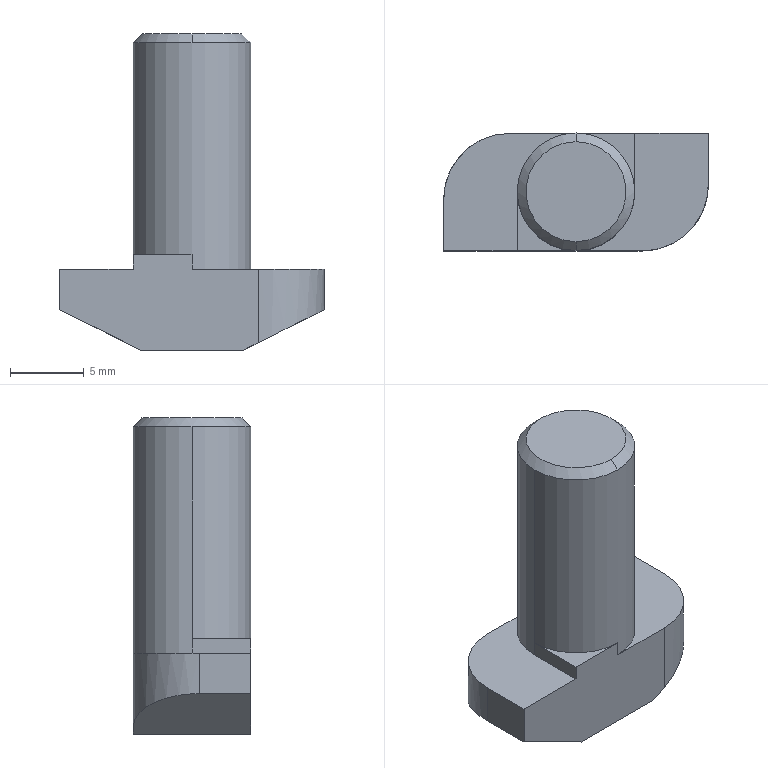Part | STEP file | LE-TS-M8X16-40_PN_0008 | 1 solid | 20 faces | box 18 x 8 x 21.5 mm | volume 1450 mm3 | plane 14 | cylinder 4 | cone 2 | commonest cylinder face diameters 8 x2 9 x2
STEP:
#1=CARTESIAN_POINT('',(0.,4.,15.4));
#2=VERTEX_POINT('',#1);
#3=CARTESIAN_POINT('',(4.,0.,15.4));
#4=VERTEX_POINT('',#3);
#5=CARTESIAN_POINT('',(0.,0.,15.4));
#6=DIRECTION('',(0.,0.,-1.));
#7=DIRECTION('',(-1.,0.,0.));
#8=AXIS2_PLACEMENT_3D('',#5,#6,#7);
#9=CIRCLE('',#8,4.);
#10=EDGE_CURVE('',#2,#4,#9,.T.);
#11=ORIENTED_EDGE('',*,*,#10,.T.);
#12=CARTESIAN_POINT('',(4.,0.,1.));
#13=VERTEX_POINT('',#12);
#14=CARTESIAN_POINT('',(4.,0.,1.));
#15=DIRECTION('',(0.,0.,-1.));
#16=VECTOR('',#15,1000.);
#17=LINE('',#14,#16);
#18=EDGE_CURVE('',#4,#13,#17,.T.);
#19=ORIENTED_EDGE('',*,*,#18,.T.);
#20=CARTESIAN_POINT('',(0.,4.,1.));
#21=VERTEX_POINT('',#20);
#22=CARTESIAN_POINT('',(0.,0.,1.));
#23=DIRECTION('',(0.,0.,1.));
#24=DIRECTION('',(-1.,0.,0.));
#25=AXIS2_PLACEMENT_3D('',#22,#23,#24);
#26=CIRCLE('',#25,4.);
#27=EDGE_CURVE('',#13,#21,#26,.T.);
#28=ORIENTED_EDGE('',*,*,#27,.T.);
#29=CARTESIAN_POINT('',(0.,4.,0.));
#30=VERTEX_POINT('',#29);
#31=CARTESIAN_POINT('',(0.,4.,0.));
#32=DIRECTION('',(0.,0.,-1.));
#33=VECTOR('',#32,1000.);
#34=LINE('',#31,#33);
#35=EDGE_CURVE('',#21,#30,#34,.T.);
#36=ORIENTED_EDGE('',*,*,#35,.T.);
#37=CARTESIAN_POINT('',(-4.,0.,0.));
#38=VERTEX_POINT('',#37);
#39=CARTESIAN_POINT('',(0.,0.,0.));
#40=DIRECTION('',(0.,0.,1.));
#41=DIRECTION('',(-1.,0.,0.));
#42=AXIS2_PLACEMENT_3D('',#39,#40,#41);
#43=CIRCLE('',#42,4.);
#44=EDGE_CURVE('',#30,#38,#43,.T.);
#45=ORIENTED_EDGE('',*,*,#44,.T.);
#46=CARTESIAN_POINT('',(-4.,0.,1.));
#47=VERTEX_POINT('',#46);
#48=CARTESIAN_POINT('',(-4.,0.,1.));
#49=DIRECTION('',(0.,0.,1.));
#50=VECTOR('',#49,1000.);
#51=LINE('',#48,#50);
#52=EDGE_CURVE('',#38,#47,#51,.T.);
#53=ORIENTED_EDGE('',*,*,#52,.T.);
#54=CARTESIAN_POINT('',(-4.,0.,15.4));
#55=VERTEX_POINT('',#54);
#56=CARTESIAN_POINT('',(-4.,0.,1.));
#57=DIRECTION('',(0.,0.,-1.));
#58=VECTOR('',#57,1000.);
#59=LINE('',#56,#58);
#60=EDGE_CURVE('',#55,#47,#59,.T.);
#61=ORIENTED_EDGE('',*,*,#60,.F.);
#62=CARTESIAN_POINT('',(0.,0.,15.4));
#63=DIRECTION('',(0.,0.,-1.));
#64=DIRECTION('',(-1.,0.,0.));
#65=AXIS2_PLACEMENT_3D('',#62,#63,#64);
#66=CIRCLE('',#65,4.);
#67=EDGE_CURVE('',#55,#2,#66,.T.);
#68=ORIENTED_EDGE('',*,*,#67,.T.);
#69=EDGE_LOOP('',(#11,#19,#28,#36,#45,#53,#61,#68));
#70=FACE_OUTER_BOUND('',#69,.T.);
#71=CARTESIAN_POINT('',(0.,0.,1.));
#72=DIRECTION('',(0.,0.,-1.));
#73=DIRECTION('',(-1.,0.,0.));
#74=AXIS2_PLACEMENT_3D('',#71,#72,#73);
#75=CYLINDRICAL_SURFACE('',#74,4.);
#76=ADVANCED_FACE('',(#70),#75,.T.);
#77=CARTESIAN_POINT('',(0.,3.4,16.));
#78=VERTEX_POINT('',#77);
#79=CARTESIAN_POINT('',(0.,-3.4,16.));
#80=VERTEX_POINT('',#79);
#81=CARTESIAN_POINT('',(0.,0.,16.));
#82=DIRECTION('',(0.,0.,-1.));
#83=DIRECTION('',(0.,1.,0.));
#84=AXIS2_PLACEMENT_3D('',#81,#82,#83);
#85=CIRCLE('',#84,3.4);
#86=EDGE_CURVE('',#78,#80,#85,.T.);
#87=ORIENTED_EDGE('',*,*,#86,.T.);
#88=CARTESIAN_POINT('',(0.,-4.,15.4));
#89=VERTEX_POINT('',#88);
#90=CARTESIAN_POINT('',(0.,-4.,15.4));
#91=DIRECTION('',(0.,-0.7071,-0.7071));
#92=VECTOR('',#91,1000.);
#93=LINE('',#90,#92);
#94=EDGE_CURVE('',#80,#89,#93,.T.);
#95=ORIENTED_EDGE('',*,*,#94,.T.);
#96=CARTESIAN_POINT('',(0.,0.,15.4));
#97=DIRECTION('',(0.,0.,-1.));
#98=DIRECTION('',(-1.,0.,0.));
#99=AXIS2_PLACEMENT_3D('',#96,#97,#98);
#100=CIRCLE('',#99,4.);
#101=EDGE_CURVE('',#4,#89,#100,.T.);
#102=ORIENTED_EDGE('',*,*,#101,.F.);
#103=ORIENTED_EDGE('',*,*,#10,.F.);
#104=CARTESIAN_POINT('',(0.,4.,15.4));
#105=DIRECTION('',(0.,0.7071,-0.7071));
#106=VECTOR('',#105,1000.);
#107=LINE('',#104,#106);
#108=EDGE_CURVE('',#78,#2,#107,.T.);
#109=ORIENTED_EDGE('',*,*,#108,.F.);
#110=EDGE_LOOP('',(#87,#95,#102,#103,#109));
#111=FACE_OUTER_BOUND('',#110,.T.);
#112=CARTESIAN_POINT('',(0.,0.,15.4));
#113=DIRECTION('',(0.,0.,-1.));
#114=DIRECTION('',(0.,1.,0.));
#115=AXIS2_PLACEMENT_3D('',#112,#113,#114);
#116=CONICAL_SURFACE('',#115,4.,0.7854);
#117=ADVANCED_FACE('',(#111),#116,.T.);
#118=ORIENTED_EDGE('',*,*,#18,.F.);
#119=ORIENTED_EDGE('',*,*,#101,.T.);
#120=CARTESIAN_POINT('',(0.,0.,15.4));
#121=DIRECTION('',(0.,0.,-1.));
#122=DIRECTION('',(-1.,0.,0.));
#123=AXIS2_PLACEMENT_3D('',#120,#121,#122);
#124=CIRCLE('',#123,4.);
#125=EDGE_CURVE('',#89,#55,#124,.T.);
#126=ORIENTED_EDGE('',*,*,#125,.T.);
#127=ORIENTED_EDGE('',*,*,#60,.T.);
#128=CARTESIAN_POINT('',(0.,-4.,1.));
#129=VERTEX_POINT('',#128);
#130=CARTESIAN_POINT('',(0.,0.,1.));
#131=DIRECTION('',(0.,0.,1.));
#132=DIRECTION('',(-1.,0.,0.));
#133=AXIS2_PLACEMENT_3D('',#130,#131,#132);
#134=CIRCLE('',#133,4.);
#135=EDGE_CURVE('',#47,#129,#134,.T.);
#136=ORIENTED_EDGE('',*,*,#135,.T.);
#137=CARTESIAN_POINT('',(0.,-4.,0.));
#138=VERTEX_POINT('',#137);
#139=CARTESIAN_POINT('',(0.,-4.,0.));
#140=DIRECTION('',(0.,0.,-1.));
#141=VECTOR('',#140,1000.);
#142=LINE('',#139,#141);
#143=EDGE_CURVE('',#129,#138,#142,.T.);
#144=ORIENTED_EDGE('',*,*,#143,.T.);
#145=CARTESIAN_POINT('',(4.,0.,0.));
#146=VERTEX_POINT('',#145);
#147=CARTESIAN_POINT('',(0.,0.,0.));
#148=DIRECTION('',(0.,0.,1.));
#149=DIRECTION('',(-1.,0.,0.));
#150=AXIS2_PLACEMENT_3D('',#147,#148,#149);
#151=CIRCLE('',#150,4.);
#152=EDGE_CURVE('',#138,#146,#151,.T.);
#153=ORIENTED_EDGE('',*,*,#152,.T.);
#154=CARTESIAN_POINT('',(4.,0.,1.));
#155=DIRECTION('',(0.,0.,1.));
#156=VECTOR('',#155,1000.);
#157=LINE('',#154,#156);
#158=EDGE_CURVE('',#146,#13,#157,.T.);
#159=ORIENTED_EDGE('',*,*,#158,.T.);
#160=EDGE_LOOP('',(#118,#119,#126,#127,#136,#144,#153,#159));
#161=FACE_OUTER_BOUND('',#160,.T.);
#162=CARTESIAN_POINT('',(0.,0.,1.));
#163=DIRECTION('',(0.,0.,-1.));
#164=DIRECTION('',(-1.,0.,0.));
#165=AXIS2_PLACEMENT_3D('',#162,#163,#164);
#166=CYLINDRICAL_SURFACE('',#165,4.);
#167=ADVANCED_FACE('',(#161),#166,.T.);
#168=CARTESIAN_POINT('',(-4.,-4.,0.));
#169=VERTEX_POINT('',#168);
#170=CARTESIAN_POINT('',(-4.,0.,0.));
#171=DIRECTION('',(0.,1.,0.));
#172=VECTOR('',#171,1000.);
#173=LINE('',#170,#172);
#174=EDGE_CURVE('',#169,#38,#173,.T.);
#175=ORIENTED_EDGE('',*,*,#174,.T.);
#176=ORIENTED_EDGE('',*,*,#44,.F.);
#177=CARTESIAN_POINT('',(-4.5,4.,0.));
#178=VERTEX_POINT('',#177);
#179=CARTESIAN_POINT('',(0.,4.,0.));
#180=DIRECTION('',(-1.,0.,0.));
#181=VECTOR('',#180,1000.);
#182=LINE('',#179,#181);
#183=EDGE_CURVE('',#30,#178,#182,.T.);
#184=ORIENTED_EDGE('',*,*,#183,.T.);
#185=CARTESIAN_POINT('',(-9.,-0.5,0.));
#186=VERTEX_POINT('',#185);
#187=CARTESIAN_POINT('',(-4.5,-0.5,0.));
#188=DIRECTION('',(0.,0.,1.));
#189=DIRECTION('',(-1.,0.,0.));
#190=AXIS2_PLACEMENT_3D('',#187,#188,#189);
#191=CIRCLE('',#190,4.5);
#192=EDGE_CURVE('',#178,#186,#191,.T.);
#193=ORIENTED_EDGE('',*,*,#192,.T.);
#194=CARTESIAN_POINT('',(-9.,-4.,0.));
#195=VERTEX_POINT('',#194);
#196=CARTESIAN_POINT('',(-9.,0.,0.));
#197=DIRECTION('',(0.,-1.,0.));
#198=VECTOR('',#197,1000.);
#199=LINE('',#196,#198);
#200=EDGE_CURVE('',#186,#195,#199,.T.);
#201=ORIENTED_EDGE('',*,*,#200,.T.);
#202=CARTESIAN_POINT('',(0.,-4.,0.));
#203=DIRECTION('',(1.,0.,0.));
#204=VECTOR('',#203,1000.);
#205=LINE('',#202,#204);
#206=EDGE_CURVE('',#195,#169,#205,.T.);
#207=ORIENTED_EDGE('',*,*,#206,.T.);
#208=EDGE_LOOP('',(#175,#176,#184,#193,#201,#207));
#209=FACE_OUTER_BOUND('',#208,.T.);
#210=CARTESIAN_POINT('',(0.,0.,0.));
#211=DIRECTION('',(0.,0.,1.));
#212=DIRECTION('',(1.,0.,0.));
#213=AXIS2_PLACEMENT_3D('',#210,#211,#212);
#214=PLANE('',#213);
#215=ADVANCED_FACE('',(#209),#214,.T.);
#216=CARTESIAN_POINT('',(4.,4.,1.));
#217=VERTEX_POINT('',#216);
#218=CARTESIAN_POINT('',(4.,0.,1.));
#219=DIRECTION('',(0.,-1.,0.));
#220=VECTOR('',#219,1000.);
#221=LINE('',#218,#220);
#222=EDGE_CURVE('',#217,#13,#221,.T.);
#223=ORIENTED_EDGE('',*,*,#222,.F.);
#224=CARTESIAN_POINT('',(0.,4.,1.));
#225=DIRECTION('',(1.,0.,0.));
#226=VECTOR('',#225,1000.);
#227=LINE('',#224,#226);
#228=EDGE_CURVE('',#21,#217,#227,.T.);
#229=ORIENTED_EDGE('',*,*,#228,.F.);
#230=ORIENTED_EDGE('',*,*,#27,.F.);
#231=EDGE_LOOP('',(#223,#229,#230));
#232=FACE_OUTER_BOUND('',#231,.T.);
#233=CARTESIAN_POINT('',(0.,0.,1.));
#234=DIRECTION('',(0.,0.,-1.));
#235=DIRECTION('',(-1.,0.,0.));
#236=AXIS2_PLACEMENT_3D('',#233,#234,#235);
#237=PLANE('',#236);
#238=ADVANCED_FACE('',(#232),#237,.F.);
#239=ORIENTED_EDGE('',*,*,#94,.F.);
#240=CARTESIAN_POINT('',(0.,0.,16.));
#241=DIRECTION('',(0.,0.,-1.));
#242=DIRECTION('',(0.,1.,0.));
#243=AXIS2_PLACEMENT_3D('',#240,#241,#242);
#244=CIRCLE('',#243,3.4);
#245=EDGE_CURVE('',#80,#78,#244,.T.);
#246=ORIENTED_EDGE('',*,*,#245,.T.);
#247=ORIENTED_EDGE('',*,*,#108,.T.);
#248=ORIENTED_EDGE('',*,*,#67,.F.);
#249=ORIENTED_EDGE('',*,*,#125,.F.);
#250=EDGE_LOOP('',(#239,#246,#247,#248,#249));
#251=FACE_OUTER_BOUND('',#250,.T.);
#252=CARTESIAN_POINT('',(0.,0.,15.4));
#253=DIRECTION('',(0.,0.,-1.));
#254=DIRECTION('',(0.,1.,0.));
#255=AXIS2_PLACEMENT_3D('',#252,#253,#254);
#256=CONICAL_SURFACE('',#255,4.,0.7854);
#257=ADVANCED_FACE('',(#251),#256,.T.);
#258=CARTESIAN_POINT('',(4.,4.,0.));
#259=VERTEX_POINT('',#258);
#260=CARTESIAN_POINT('',(4.,0.,0.));
#261=DIRECTION('',(0.,-1.,0.));
#262=VECTOR('',#261,1000.);
#263=LINE('',#260,#262);
#264=EDGE_CURVE('',#259,#146,#263,.T.);
#265=ORIENTED_EDGE('',*,*,#264,.T.);
#266=ORIENTED_EDGE('',*,*,#152,.F.);
#267=CARTESIAN_POINT('',(4.5,-4.,0.));
#268=VERTEX_POINT('',#267);
#269=CARTESIAN_POINT('',(0.,-4.,0.));
#270=DIRECTION('',(1.,0.,0.));
#271=VECTOR('',#270,1000.);
#272=LINE('',#269,#271);
#273=EDGE_CURVE('',#138,#268,#272,.T.);
#274=ORIENTED_EDGE('',*,*,#273,.T.);
#275=CARTESIAN_POINT('',(9.,0.5,0.));
#276=VERTEX_POINT('',#275);
#277=CARTESIAN_POINT('',(4.5,0.5,0.));
#278=DIRECTION('',(0.,0.,1.));
#279=DIRECTION('',(-1.,0.,0.));
#280=AXIS2_PLACEMENT_3D('',#277,#278,#279);
#281=CIRCLE('',#280,4.5);
#282=EDGE_CURVE('',#268,#276,#281,.T.);
#283=ORIENTED_EDGE('',*,*,#282,.T.);
#284=CARTESIAN_POINT('',(9.,4.,0.));
#285=VERTEX_POINT('',#284);
#286=CARTESIAN_POINT('',(9.,0.,0.));
#287=DIRECTION('',(0.,1.,0.));
#288=VECTOR('',#287,1000.);
#289=LINE('',#286,#288);
#290=EDGE_CURVE('',#276,#285,#289,.T.);
#291=ORIENTED_EDGE('',*,*,#290,.T.);
#292=CARTESIAN_POINT('',(0.,4.,0.));
#293=DIRECTION('',(-1.,0.,0.));
#294=VECTOR('',#293,1000.);
#295=LINE('',#292,#294);
#296=EDGE_CURVE('',#285,#259,#295,.T.);
#297=ORIENTED_EDGE('',*,*,#296,.T.);
#298=EDGE_LOOP('',(#265,#266,#274,#283,#291,#297));
#299=FACE_OUTER_BOUND('',#298,.T.);
#300=CARTESIAN_POINT('',(0.,0.,0.));
#301=DIRECTION('',(0.,0.,1.));
#302=DIRECTION('',(1.,0.,0.));
#303=AXIS2_PLACEMENT_3D('',#300,#301,#302);
#304=PLANE('',#303);
#305=ADVANCED_FACE('',(#299),#304,.T.);
#306=CARTESIAN_POINT('',(-4.,-4.,1.));
#307=VERTEX_POINT('',#306);
#308=CARTESIAN_POINT('',(-4.,0.,1.));
#309=DIRECTION('',(0.,1.,0.));
#310=VECTOR('',#309,1000.);
#311=LINE('',#308,#310);
#312=EDGE_CURVE('',#307,#47,#311,.T.);
#313=ORIENTED_EDGE('',*,*,#312,.F.);
#314=CARTESIAN_POINT('',(0.,-4.,1.));
#315=DIRECTION('',(-1.,0.,0.));
#316=VECTOR('',#315,1000.);
#317=LINE('',#314,#316);
#318=EDGE_CURVE('',#129,#307,#317,.T.);
#319=ORIENTED_EDGE('',*,*,#318,.F.);
#320=ORIENTED_EDGE('',*,*,#135,.F.);
#321=EDGE_LOOP('',(#313,#319,#320));
#322=FACE_OUTER_BOUND('',#321,.T.);
#323=CARTESIAN_POINT('',(0.,0.,1.));
#324=DIRECTION('',(0.,0.,-1.));
#325=DIRECTION('',(-1.,0.,0.));
#326=AXIS2_PLACEMENT_3D('',#323,#324,#325);
#327=PLANE('',#326);
#328=ADVANCED_FACE('',(#322),#327,.F.);
#329=ORIENTED_EDGE('',*,*,#52,.F.);
#330=ORIENTED_EDGE('',*,*,#174,.F.);
#331=CARTESIAN_POINT('',(-4.,-4.,1.));
#332=DIRECTION('',(0.,0.,-1.));
#333=VECTOR('',#332,1000.);
#334=LINE('',#331,#333);
#335=EDGE_CURVE('',#307,#169,#334,.T.);
#336=ORIENTED_EDGE('',*,*,#335,.F.);
#337=ORIENTED_EDGE('',*,*,#312,.T.);
#338=EDGE_LOOP('',(#329,#330,#336,#337));
#339=FACE_OUTER_BOUND('',#338,.T.);
#340=CARTESIAN_POINT('',(-4.,-4.,1.));
#341=DIRECTION('',(1.,0.,0.));
#342=DIRECTION('',(0.,0.,-1.));
#343=AXIS2_PLACEMENT_3D('',#340,#341,#342);
#344=PLANE('',#343);
#345=ADVANCED_FACE('',(#339),#344,.F.);
#346=CARTESIAN_POINT('',(4.5,-4.,-5.));
#347=VERTEX_POINT('',#346);
#348=CARTESIAN_POINT('',(4.5,-4.,0.));
#349=DIRECTION('',(0.,0.,-1.));
#350=VECTOR('',#349,1000.);
#351=LINE('',#348,#350);
#352=EDGE_CURVE('',#268,#347,#351,.T.);
#353=ORIENTED_EDGE('',*,*,#352,.F.);
#354=ORIENTED_EDGE('',*,*,#273,.F.);
#355=ORIENTED_EDGE('',*,*,#143,.F.);
#356=ORIENTED_EDGE('',*,*,#318,.T.);
#357=ORIENTED_EDGE('',*,*,#335,.T.);
#358=ORIENTED_EDGE('',*,*,#206,.F.);
#359=CARTESIAN_POINT('',(-9.,-4.,-2.75));
#360=VERTEX_POINT('',#359);
#361=CARTESIAN_POINT('',(-9.,-4.,0.));
#362=DIRECTION('',(0.,0.,1.));
#363=VECTOR('',#362,1000.);
#364=LINE('',#361,#363);
#365=EDGE_CURVE('',#360,#195,#364,.T.);
#366=ORIENTED_EDGE('',*,*,#365,.F.);
#367=CARTESIAN_POINT('',(-3.5,-4.,-5.5));
#368=VERTEX_POINT('',#367);
#369=CARTESIAN_POINT('',(-3.5,-4.,-5.5));
#370=DIRECTION('',(-0.8944,0.,0.4472));
#371=VECTOR('',#370,1000.);
#372=LINE('',#369,#371);
#373=EDGE_CURVE('',#368,#360,#372,.T.);
#374=ORIENTED_EDGE('',*,*,#373,.F.);
#375=CARTESIAN_POINT('',(3.5,-4.,-5.5));
#376=VERTEX_POINT('',#375);
#377=CARTESIAN_POINT('',(-9.,-4.,-5.5));
#378=DIRECTION('',(-1.,0.,0.));
#379=VECTOR('',#378,1000.);
#380=LINE('',#377,#379);
#381=EDGE_CURVE('',#376,#368,#380,.T.);
#382=ORIENTED_EDGE('',*,*,#381,.F.);
#383=CARTESIAN_POINT('',(9.,-4.,-2.75));
#384=DIRECTION('',(0.8944,0.,0.4472));
#385=VECTOR('',#384,1000.);
#386=LINE('',#383,#385);
#387=EDGE_CURVE('',#376,#347,#386,.T.);
#388=ORIENTED_EDGE('',*,*,#387,.T.);
#389=EDGE_LOOP('',(#353,#354,#355,#356,#357,#358,#366,#374,#382,#388));
#390=FACE_OUTER_BOUND('',#389,.T.);
#391=CARTESIAN_POINT('',(-9.,-4.,0.));
#392=DIRECTION('',(0.,1.,0.));
#393=DIRECTION('',(0.,0.,1.));
#394=AXIS2_PLACEMENT_3D('',#391,#392,#393);
#395=PLANE('',#394);
#396=ADVANCED_FACE('',(#390),#395,.F.);
#397=CARTESIAN_POINT('',(-9.,-0.5,-2.75));
#398=VERTEX_POINT('',#397);
#399=CARTESIAN_POINT('',(-9.,-0.5,0.));
#400=DIRECTION('',(0.,0.,1.));
#401=VECTOR('',#400,1000.);
#402=LINE('',#399,#401);
#403=EDGE_CURVE('',#398,#186,#402,.T.);
#404=ORIENTED_EDGE('',*,*,#403,.F.);
#405=CARTESIAN_POINT('',(-9.,4.,-2.75));
#406=DIRECTION('',(0.,1.,0.));
#407=VECTOR('',#406,1000.);
#408=LINE('',#405,#407);
#409=EDGE_CURVE('',#360,#398,#408,.T.);
#410=ORIENTED_EDGE('',*,*,#409,.F.);
#411=ORIENTED_EDGE('',*,*,#365,.T.);
#412=ORIENTED_EDGE('',*,*,#200,.F.);
#413=EDGE_LOOP('',(#404,#410,#411,#412));
#414=FACE_OUTER_BOUND('',#413,.T.);
#415=CARTESIAN_POINT('',(-9.,4.,0.));
#416=DIRECTION('',(1.,0.,0.));
#417=DIRECTION('',(0.,0.,-1.));
#418=AXIS2_PLACEMENT_3D('',#415,#416,#417);
#419=PLANE('',#418);
#420=ADVANCED_FACE('',(#414),#419,.F.);
#421=CARTESIAN_POINT('',(-4.5,4.,-5.));
#422=VERTEX_POINT('',#421);
#423=CARTESIAN_POINT('',(-4.5,4.,-5.));
#424=CARTESIAN_POINT('',(-7.136,4.,-3.682));
#425=CARTESIAN_POINT('',(-9.,2.136,-2.75));
#426=CARTESIAN_POINT('',(-9.,-0.5,-2.75));
#427=(BOUNDED_CURVE()B_SPLINE_CURVE(3,(#423,#424,#425,#426),.UNSPECIFIED.,.F.,.T.)B_SPLINE_CURVE_WITH_KNOTS((4,4),(1.571,3.142),.UNSPECIFIED.)CURVE()GEOMETRIC_REPRESENTATION_ITEM()RATIONAL_B_SPLINE_CURVE((1.,0.8047,0.8047,1.))REPRESENTATION_ITEM(''));
#428=EDGE_CURVE('',#422,#398,#427,.T.);
#429=ORIENTED_EDGE('',*,*,#428,.T.);
#430=ORIENTED_EDGE('',*,*,#403,.T.);
#431=ORIENTED_EDGE('',*,*,#192,.F.);
#432=CARTESIAN_POINT('',(-4.5,4.,0.));
#433=DIRECTION('',(0.,0.,-1.));
#434=VECTOR('',#433,1000.);
#435=LINE('',#432,#434);
#436=EDGE_CURVE('',#178,#422,#435,.T.);
#437=ORIENTED_EDGE('',*,*,#436,.T.);
#438=EDGE_LOOP('',(#429,#430,#431,#437));
#439=FACE_OUTER_BOUND('',#438,.T.);
#440=CARTESIAN_POINT('',(-4.5,-0.5,0.));
#441=DIRECTION('',(0.,0.,-1.));
#442=DIRECTION('',(-1.,0.,0.));
#443=AXIS2_PLACEMENT_3D('',#440,#441,#442);
#444=CYLINDRICAL_SURFACE('',#443,4.5);
#445=ADVANCED_FACE('',(#439),#444,.T.);
#446=ORIENTED_EDGE('',*,*,#436,.F.);
#447=ORIENTED_EDGE('',*,*,#183,.F.);
#448=ORIENTED_EDGE('',*,*,#35,.F.);
#449=ORIENTED_EDGE('',*,*,#228,.T.);
#450=CARTESIAN_POINT('',(4.,4.,0.));
#451=DIRECTION('',(0.,0.,1.));
#452=VECTOR('',#451,1000.);
#453=LINE('',#450,#452);
#454=EDGE_CURVE('',#259,#217,#453,.T.);
#455=ORIENTED_EDGE('',*,*,#454,.F.);
#456=ORIENTED_EDGE('',*,*,#296,.F.);
#457=CARTESIAN_POINT('',(9.,4.,-2.75));
#458=VERTEX_POINT('',#457);
#459=CARTESIAN_POINT('',(9.,4.,0.));
#460=DIRECTION('',(0.,0.,1.));
#461=VECTOR('',#460,1000.);
#462=LINE('',#459,#461);
#463=EDGE_CURVE('',#458,#285,#462,.T.);
#464=ORIENTED_EDGE('',*,*,#463,.F.);
#465=CARTESIAN_POINT('',(3.5,4.,-5.5));
#466=VERTEX_POINT('',#465);
#467=CARTESIAN_POINT('',(3.5,4.,-5.5));
#468=DIRECTION('',(0.8944,0.,0.4472));
#469=VECTOR('',#468,1000.);
#470=LINE('',#467,#469);
#471=EDGE_CURVE('',#466,#458,#470,.T.);
#472=ORIENTED_EDGE('',*,*,#471,.F.);
#473=CARTESIAN_POINT('',(-3.5,4.,-5.5));
#474=VERTEX_POINT('',#473);
#475=CARTESIAN_POINT('',(-9.,4.,-5.5));
#476=DIRECTION('',(1.,0.,0.));
#477=VECTOR('',#476,1000.);
#478=LINE('',#475,#477);
#479=EDGE_CURVE('',#474,#466,#478,.T.);
#480=ORIENTED_EDGE('',*,*,#479,.F.);
#481=CARTESIAN_POINT('',(-4.5,4.,-5.));
#482=DIRECTION('',(0.8944,0.,-0.4472));
#483=VECTOR('',#482,1000.);
#484=LINE('',#481,#483);
#485=EDGE_CURVE('',#422,#474,#484,.T.);
#486=ORIENTED_EDGE('',*,*,#485,.F.);
#487=EDGE_LOOP('',(#446,#447,#448,#449,#455,#456,#464,#472,#480,#486));
#488=FACE_OUTER_BOUND('',#487,.T.);
#489=CARTESIAN_POINT('',(-9.,4.,0.));
#490=DIRECTION('',(0.,-1.,0.));
#491=DIRECTION('',(0.,0.,-1.));
#492=AXIS2_PLACEMENT_3D('',#489,#490,#491);
#493=PLANE('',#492);
#494=ADVANCED_FACE('',(#488),#493,.F.);
#495=ORIENTED_EDGE('',*,*,#158,.F.);
#496=ORIENTED_EDGE('',*,*,#264,.F.);
#497=ORIENTED_EDGE('',*,*,#454,.T.);
#498=ORIENTED_EDGE('',*,*,#222,.T.);
#499=EDGE_LOOP('',(#495,#496,#497,#498));
#500=FACE_OUTER_BOUND('',#499,.T.);
#501=CARTESIAN_POINT('',(4.,-4.,1.));
#502=DIRECTION('',(-1.,0.,0.));
#503=DIRECTION('',(0.,0.,1.));
#504=AXIS2_PLACEMENT_3D('',#501,#502,#503);
#505=PLANE('',#504);
#506=ADVANCED_FACE('',(#500),#505,.F.);
#507=ORIENTED_EDGE('',*,*,#86,.F.);
#508=ORIENTED_EDGE('',*,*,#245,.F.);
#509=EDGE_LOOP('',(#507,#508));
#510=FACE_OUTER_BOUND('',#509,.T.);
#511=CARTESIAN_POINT('',(0.,0.,16.));
#512=DIRECTION('',(0.,0.,1.));
#513=DIRECTION('',(1.,0.,0.));
#514=AXIS2_PLACEMENT_3D('',#511,#512,#513);
#515=PLANE('',#514);
#516=ADVANCED_FACE('',(#510),#515,.T.);
#517=CARTESIAN_POINT('',(9.,0.5,-2.75));
#518=VERTEX_POINT('',#517);
#519=CARTESIAN_POINT('',(9.,0.5,0.));
#520=DIRECTION('',(0.,0.,1.));
#521=VECTOR('',#520,1000.);
#522=LINE('',#519,#521);
#523=EDGE_CURVE('',#518,#276,#522,.T.);
#524=ORIENTED_EDGE('',*,*,#523,.F.);
#525=CARTESIAN_POINT('',(9.,4.,-2.75));
#526=DIRECTION('',(0.,-1.,0.));
#527=VECTOR('',#526,1000.);
#528=LINE('',#525,#527);
#529=EDGE_CURVE('',#458,#518,#528,.T.);
#530=ORIENTED_EDGE('',*,*,#529,.F.);
#531=ORIENTED_EDGE('',*,*,#463,.T.);
#532=ORIENTED_EDGE('',*,*,#290,.F.);
#533=EDGE_LOOP('',(#524,#530,#531,#532));
#534=FACE_OUTER_BOUND('',#533,.T.);
#535=CARTESIAN_POINT('',(9.,4.,0.));
#536=DIRECTION('',(-1.,0.,0.));
#537=DIRECTION('',(0.,0.,1.));
#538=AXIS2_PLACEMENT_3D('',#535,#536,#537);
#539=PLANE('',#538);
#540=ADVANCED_FACE('',(#534),#539,.F.);
#541=CARTESIAN_POINT('',(4.5,-4.,-5.));
#542=CARTESIAN_POINT('',(7.136,-4.,-3.682));
#543=CARTESIAN_POINT('',(9.,-2.136,-2.75));
#544=CARTESIAN_POINT('',(9.,0.5,-2.75));
#545=(BOUNDED_CURVE()B_SPLINE_CURVE(3,(#541,#542,#543,#544),.UNSPECIFIED.,.F.,.T.)B_SPLINE_CURVE_WITH_KNOTS((4,4),(1.571,3.142),.UNSPECIFIED.)CURVE()GEOMETRIC_REPRESENTATION_ITEM()RATIONAL_B_SPLINE_CURVE((1.,0.8047,0.8047,1.))REPRESENTATION_ITEM(''));
#546=EDGE_CURVE('',#347,#518,#545,.T.);
#547=ORIENTED_EDGE('',*,*,#546,.T.);
#548=ORIENTED_EDGE('',*,*,#523,.T.);
#549=ORIENTED_EDGE('',*,*,#282,.F.);
#550=ORIENTED_EDGE('',*,*,#352,.T.);
#551=EDGE_LOOP('',(#547,#548,#549,#550));
#552=FACE_OUTER_BOUND('',#551,.T.);
#553=CARTESIAN_POINT('',(4.5,0.5,0.));
#554=DIRECTION('',(0.,0.,-1.));
#555=DIRECTION('',(-1.,0.,0.));
#556=AXIS2_PLACEMENT_3D('',#553,#554,#555);
#557=CYLINDRICAL_SURFACE('',#556,4.5);
#558=ADVANCED_FACE('',(#552),#557,.T.);
#559=ORIENTED_EDGE('',*,*,#428,.F.);
#560=ORIENTED_EDGE('',*,*,#485,.T.);
#561=CARTESIAN_POINT('',(-3.5,4.,-5.5));
#562=DIRECTION('',(0.,1.,0.));
#563=VECTOR('',#562,1000.);
#564=LINE('',#561,#563);
#565=EDGE_CURVE('',#368,#474,#564,.T.);
#566=ORIENTED_EDGE('',*,*,#565,.F.);
#567=ORIENTED_EDGE('',*,*,#373,.T.);
#568=ORIENTED_EDGE('',*,*,#409,.T.);
#569=EDGE_LOOP('',(#559,#560,#566,#567,#568));
#570=FACE_OUTER_BOUND('',#569,.T.);
#571=CARTESIAN_POINT('',(-9.,4.,-2.75));
#572=DIRECTION('',(0.4472,0.,0.8944));
#573=DIRECTION('',(0.8944,0.,-0.4472));
#574=AXIS2_PLACEMENT_3D('',#571,#572,#573);
#575=PLANE('',#574);
#576=ADVANCED_FACE('',(#570),#575,.F.);
#577=CARTESIAN_POINT('',(3.5,0.,-5.5));
#578=DIRECTION('',(0.,1.,0.));
#579=VECTOR('',#578,1000.);
#580=LINE('',#577,#579);
#581=EDGE_CURVE('',#376,#466,#580,.T.);
#582=ORIENTED_EDGE('',*,*,#581,.F.);
#583=ORIENTED_EDGE('',*,*,#381,.T.);
#584=ORIENTED_EDGE('',*,*,#565,.T.);
#585=ORIENTED_EDGE('',*,*,#479,.T.);
#586=EDGE_LOOP('',(#582,#583,#584,#585));
#587=FACE_OUTER_BOUND('',#586,.T.);
#588=CARTESIAN_POINT('',(0.,0.,-5.5));
#589=DIRECTION('',(0.,0.,1.));
#590=DIRECTION('',(1.,0.,0.));
#591=AXIS2_PLACEMENT_3D('',#588,#589,#590);
#592=PLANE('',#591);
#593=ADVANCED_FACE('',(#587),#592,.F.);
#594=ORIENTED_EDGE('',*,*,#546,.F.);
#595=ORIENTED_EDGE('',*,*,#387,.F.);
#596=ORIENTED_EDGE('',*,*,#581,.T.);
#597=ORIENTED_EDGE('',*,*,#471,.T.);
#598=ORIENTED_EDGE('',*,*,#529,.T.);
#599=EDGE_LOOP('',(#594,#595,#596,#597,#598));
#600=FACE_OUTER_BOUND('',#599,.T.);
#601=CARTESIAN_POINT('',(9.,4.,-2.75));
#602=DIRECTION('',(-0.4472,0.,0.8944));
#603=DIRECTION('',(0.8944,0.,0.4472));
#604=AXIS2_PLACEMENT_3D('',#601,#602,#603);
#605=PLANE('',#604);
#606=ADVANCED_FACE('',(#600),#605,.F.);
#607=CLOSED_SHELL('',(#76,#117,#167,#215,#238,#257,#305,#328,#345,#396,#420,#445,#494,#506,#516,#540,#558,#576,#593,#606));
#608=MANIFOLD_SOLID_BREP('',#607);
#609=CARTESIAN_POINT('',(0.,0.,0.));
#610=DIRECTION('',(0.,0.,1.));
#611=DIRECTION('',(1.,0.,0.));
#612=AXIS2_PLACEMENT_3D('',#609,#610,#611);
#613=(LENGTH_UNIT()NAMED_UNIT(*)SI_UNIT(.MILLI.,.METRE.));
#614=UNCERTAINTY_MEASURE_WITH_UNIT(LENGTH_MEASURE(0.00001),#613,'','');
#615=(NAMED_UNIT(*)PLANE_ANGLE_UNIT()SI_UNIT($,.RADIAN.));
#616=(NAMED_UNIT(*)SI_UNIT($,.STERADIAN.)SOLID_ANGLE_UNIT());
#617=(GEOMETRIC_REPRESENTATION_CONTEXT(3)GLOBAL_UNCERTAINTY_ASSIGNED_CONTEXT((#614))GLOBAL_UNIT_ASSIGNED_CONTEXT((#613,#615,#616))REPRESENTATION_CONTEXT('',''));
#618=ADVANCED_BREP_SHAPE_REPRESENTATION('',(#608,#612),#617);